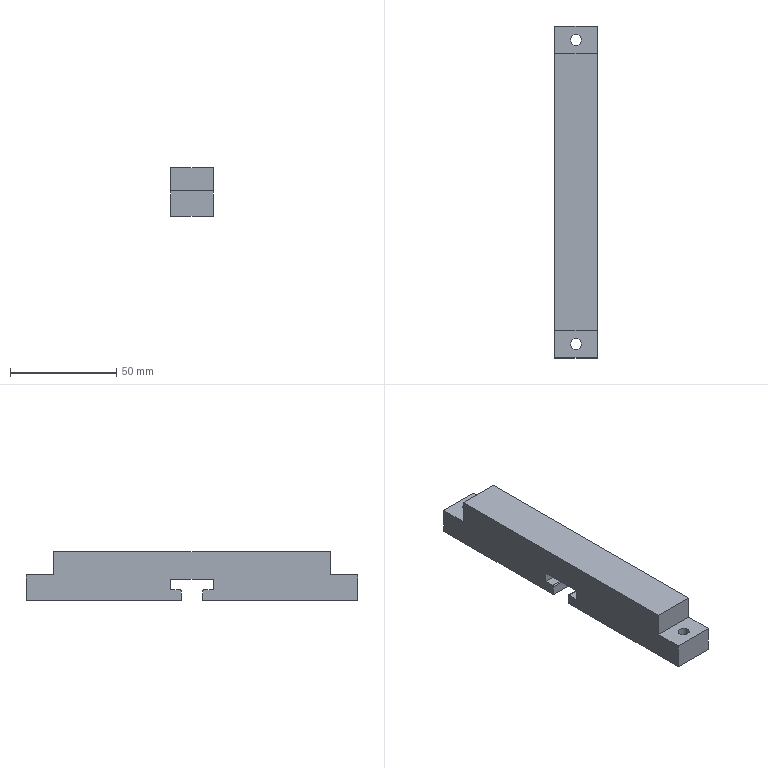Part | STEP file | 1 solid | 26 faces | box 20 x 156 x 23.01 mm | volume 61919 mm3 | plane 20 | cylinder 6 | commonest cylinder face diameters 1 x2 5.2 x2 9 x2